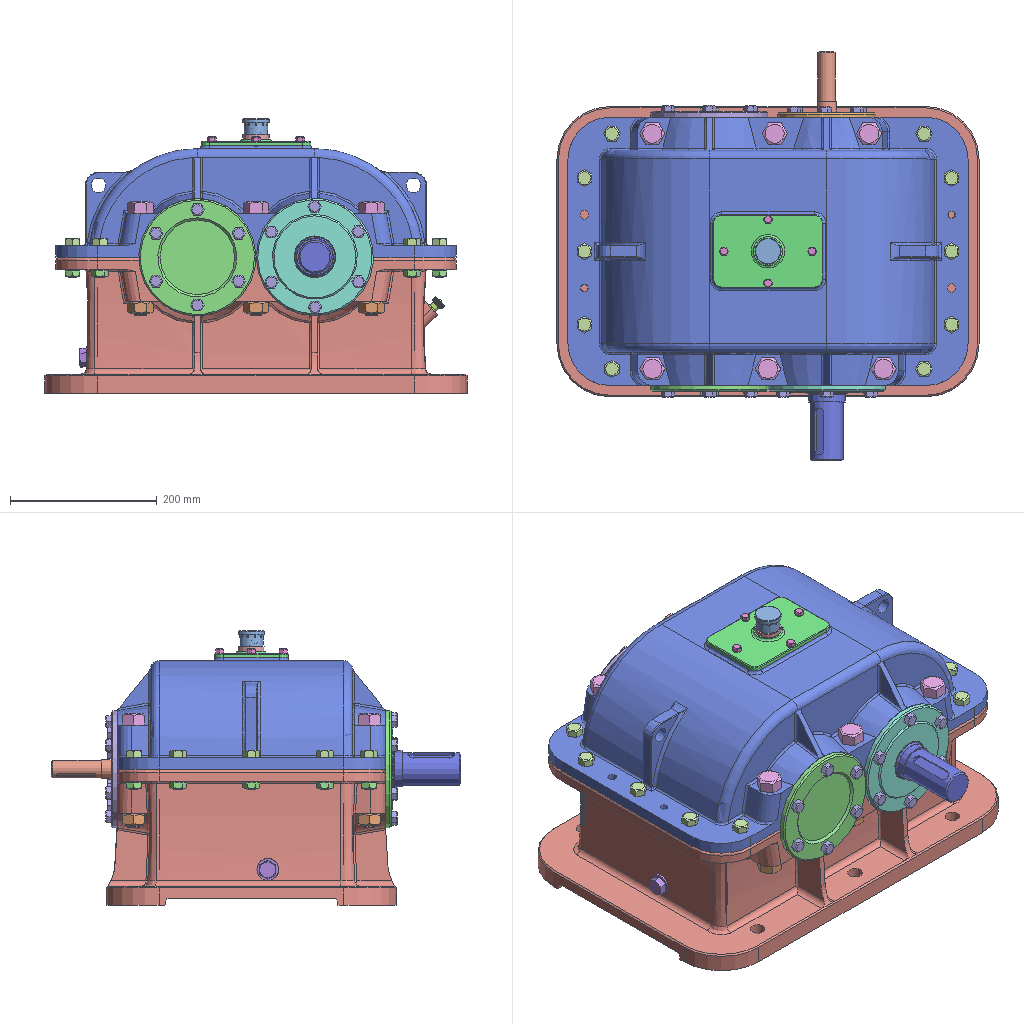Assembly | NX | 39 different items | 103 placed | box 576 x 558 x 375 mm
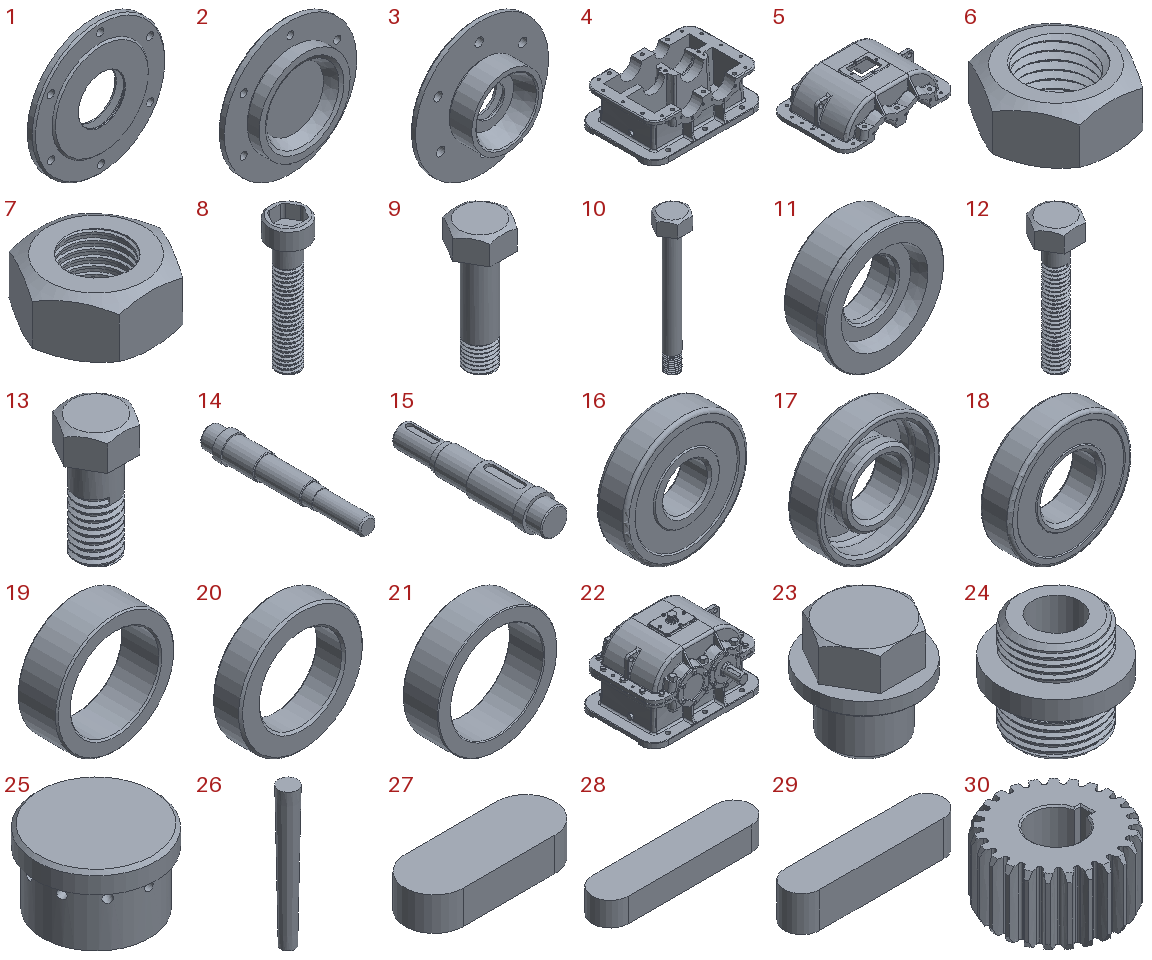Parts list (item | quantity | parent item | size | volume | features):
1 | x1 | in 22 | 160 x 18 x 160 mm | 177921 mm3 | features BREP 1, DATUM_CSYS 1
2 | x1 | in 22 | 160 x 25 x 160 mm | 214879 mm3 | features BREP 1, DATUM_CSYS 1
3 | x1 | in 22 | 135 x 31.5 x 135 mm | 118525 mm3 | features BREP 1, DATUM_CSYS 1
4 | x1 | in 22 | 576 x 396 x 186 mm | 12365991 mm3 | features DATUM_CSYS 8, SKETCH 7, EXTRUDE 6, BLEND 2, DATUM_PLANE 2, THREADS 2, BREP 1
5 | x1 | in 22 | - | - | features BLEND 4, DATUM_CSYS 3, EXTRUDE 3, SKETCH 2, BREP 1, CPROJ 1, DATUM_PLANE 1
6 | x10 | in 22 | 23.094 x 20 x 10 mm | 1985 mm3 | features DATUM_CSYS 3, SKETCH 2, EXTRUDE 1, SWP104 1, THREADS 1
7 | x6 | in 22 | 34.641 x 30 x 16 mm | 8595 mm3 | features DATUM_CSYS 3, SKETCH 2, EXTRUDE 1, SWP104 1, THREADS 1
8 | x2 | in 22 | 20 x 20 x 70 mm | 7911 mm3 | features DATUM_CSYS 3, EXTRUDE 2, SKETCH 2, BLEND 1, CHAMFER 1, CYLINDER 1, THREADS 1
9 | x10 | in 22 | - | - | features DATUM_CSYS 3, SKETCH 2, CYLINDER 1, EXTRUDE 1, SWP104 1, THREADS 1
10 | x6 | in 22 | 34.641 x 30 x 156 mm | 39944 mm3 | features DATUM_CSYS 3, SKETCH 2, CYLINDER 1, EXTRUDE 1, SWP104 1, THREADS 1
11 | x1 | in 22 | 130 x 50.5 x 130 mm | 363881 mm3 | features BREP 1, DATUM_CSYS 1
12 | x24 | in 22 | 18.475 x 16 x 56 mm | 4007 mm3 | features DATUM_CSYS 3, SKETCH 2, CYLINDER 1, EXTRUDE 1, SWP104 1, THREADS 1
13 | x4 | in 22 | - | - | features DATUM_CSYS 3, SKETCH 2, CYLINDER 1, EXTRUDE 1, SWP104 1, THREADS 1
14 | x1 | in 22 | 38 x 227.5 x 38 mm | 152701 mm3 | features DATUM_CSYS 4, SKETCH 3, CHAMFER 2, DATUM_PLANE 2, EXTRUDE 2, CPROJ 1, SWP104 1
15 | x1 | in 22 | 68 x 312 x 68 mm | 761578 mm3 | features DATUM_CSYS 4, CHAMFER 3, SKETCH 3, DATUM_PLANE 2, EXTRUDE 2, SWP104 1
16 | x2 | in 22 | 110 x 27 x 110 mm | 123017 mm3 | features BREP 1, DATUM_CSYS 1
17 | x2 | in 22 | 72 x 19 x 72 mm | 32783 mm3 | features BREP 1, DATUM_CSYS 1
18 | x2 | in 22 | 120 x 29 x 120 mm | 129024 mm3 | features BREP 1, DATUM_CSYS 1
19 | x1 | - | 40 x 13.5 x 40 mm | 7367 mm3 | features BREP 1, DATUM_CSYS 1
20 | x1 | - | 60 x 14 x 60 mm | 21677 mm3 | features BREP 1, DATUM_CSYS 1
21 | x1 | - | 71 x 21 x 71 mm | 33152 mm3 | features BREP 1, DATUM_CSYS 1
22 | x1 | - | - | 23332165 mm3 | features BREP 221, META 208, DATUM_CSYS 102, SWP104 95, EXTRACT_STRING 92, Instance Feature 88, SKETCH 68, EXTRUDE 61, CHAMFER 19, BLEND 12, CYLINDER 10, DATUM_PLANE 10, THREADS 9, CPROJ 7, BOSS 4, FSET 4, Pattern Feature 3, Mirror Feature 1, WRAP 1
23 | x1 | in 22 | 30 x 30 x 29 mm | 11364 mm3 | features DATUM_CSYS 4, SKETCH 3, CHAMFER 2, SWP104 2, DATUM_PLANE 1, EXTRUDE 1
24 | x1 | in 22 | 36 x 36 x 32 mm | 13512 mm3 | features BREP 1, DATUM_CSYS 1
25 | x1 | in 22 | 36 x 36 x 22 mm | 11377 mm3 | features EXTRUDE 12, EXTRACT_STRING 10, Instance Feature 9, DATUM_CSYS 4, SKETCH 3, BOSS 1, CHAMFER 1, CYLINDER 1, Pattern Feature 1
26 | x2 | in 22 | 8.095 x 8.095 x 60 mm | 2358 mm3 | features DATUM_CSYS 2, EXTRUDE 1, SKETCH 1
27 | x1 | in 22 | 36 x 14 x 8 mm | 3696 mm3 | features DATUM_CSYS 2, EXTRUDE 1, SKETCH 1
28 | x1 | in 22 | 80 x 18 x 12 mm | 16446 mm3 | features DATUM_CSYS 2, EXTRUDE 1, SKETCH 1
29 | x1 | in 22 | 36 x 8 x 8 mm | 2194 mm3 | features DATUM_CSYS 2, EXTRUDE 1, SKETCH 1
30 | x1 | in 22 | 83.645 x 83.495 x 45 mm | 166384 mm3 | features BREP 25, META 25, DATUM_CSYS 4, SKETCH 3, EXTRUDE 2, CHAMFER 1, CPROJ 1, CYLINDER 1, FSET 1, SWP104 1
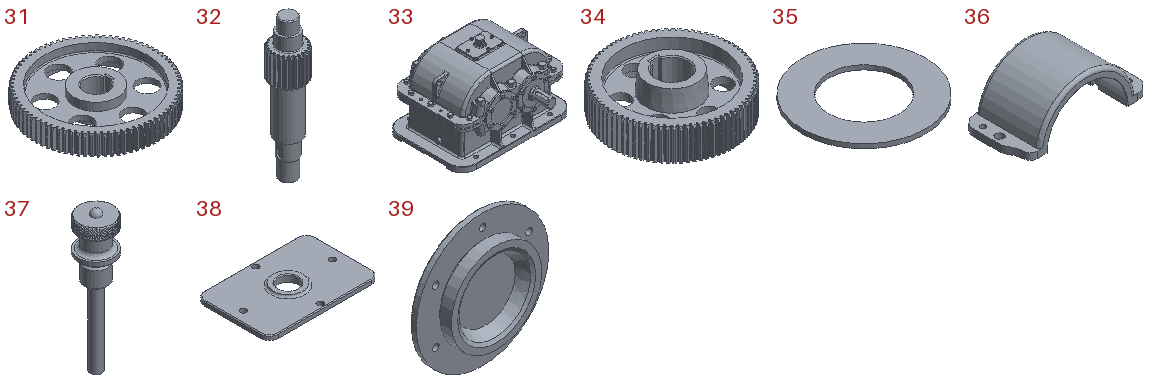31 | x1 | in 22 | 247.038 x 246.995 x 40 mm | 857249 mm3 | features BREP 79, META 79, DATUM_CSYS 7, SKETCH 6, EXTRUDE 5, CPROJ 2, BLEND 1, CHAMFER 1, CYLINDER 1, FSET 1, SWP104 1
32 | x1 | in 22 | 82.296 x 82.148 x 342.25 mm | 879629 mm3 | features BREP 25, META 25, DATUM_CSYS 5, SKETCH 4, BOSS 3, EXTRUDE 3, CHAMFER 2, BLEND 1, CYLINDER 1, FSET 1, SWP104 1
33 | x1 | - | - | 23332165 mm3 | features BREP 221, META 208, DATUM_CSYS 102, SWP104 95, EXTRACT_STRING 92, Instance Feature 88, SKETCH 68, EXTRUDE 61, CHAMFER 19, BLEND 12, CYLINDER 10, DATUM_PLANE 10, THREADS 9, CPROJ 7, BOSS 4, FSET 4, Pattern Feature 3, Mirror Feature 1, WRAP 1
34 | x1 | in 22 | 247.038 x 246.995 x 94 mm | 1592670 mm3 | features BREP 79, META 79, DATUM_CSYS 10, SKETCH 9, EXTRUDE 8, BLEND 1, CHAMFER 1, CPROJ 1, CYLINDER 1, FSET 1, SWP104 1
35 | x6 | in 22 | 28 x 28 x 1 mm | 414.69 mm3 | features DATUM_CSYS 2, EXTRUDE 1, SKETCH 1
36 | x1 | in 22 | 190 x 95 x 73.244 mm | 279574 mm3 | features BREP 1, CHAMFER 1, DATUM_CSYS 1, DATUM_PLANE 1
37 | x1 | in 22 | 18 x 18 x 72.5 mm | 5643 mm3 | features EXTRACT_STRING 82, SWP104 81, Instance Feature 79, DATUM_CSYS 4, CHAMFER 3, SKETCH 3, Pattern Feature 2, BLEND 1, DATUM_PLANE 1, Mirror Feature 1, WRAP 1
38 | x1 | in 22 | 150 x 100 x 10 mm | 75362 mm3 | features DATUM_CSYS 2, BLEND 1, BREP 1, CHAMFER 1, CPROJ 1, EXTRUDE 1, SKETCH 1
39 | x1 | in 22 | 160 x 25 x 160 mm | 214093 mm3 | features DATUM_CSYS 3, EXTRUDE 3, SKETCH 2, BREP 1
Mates (type | each side: item.copy, entity, surface, feature):
Fix | 4.1 component
Concentric | 4.1 edge | 5.1 edge
Parallel | 5.1 face plane Body(1) | 4.1 face plane Body(1)
Concentric | 3.1 edge | 5.1 edge | 2 times
Concentric | 5.1 edge | 1.1 edge | 2 times
Concentric | 5.1 edge | 39.1 edge
Distance | 39.1 face cylinder Extrude(6) | 5.1 face cylinder Body(1)
Concentric | 5.1 edge | 2.1 edge
Distance | 2.1 face cylinder Body(1) | 5.1 face cylinder Body(1)
Concentric | 11.1 edge | 4.1 edge
Concentric | 2.1 edge | 16.1 edge
Concentric | 16.1 edge | 39.1 edge
Concentric | 17.1 edge | 3.1 edge
Concentric | 1.1 edge | 18.1 edge
Concentric | 18.1 edge | 11.1 edge
Concentric | 4.1 edge | 36.1 edge
Parallel | 36.1 face plane Body(1) | 11.1 face plane Body(1)
Concentric | 17.1 edge | 11.1 edge
Touch | 14.1 face cylinder Revolve(2) | 3.1 face cylinder Body(1)
Distance | 14.1 face plane Revolve(2) | 3.1 face plane Body(1)
Touch | 15.1 face cylinder Revolve(2) | 18.1 face cone Body(1)
Distance | 15.1 face plane Revolve(2) | 1.1 face plane Body(1)
Parallel | 30.1 face plane Extrude(56) | 14.1 face plane Extrude(7)
Touch | 30.1 face cylinder Extrude(54) | 14.1 face cylinder Revolve(2)
Center22 | 30.1 face plane Cylinder(1) | 30.1 face plane Cylinder(1) | 4.1 face plane Body(1) | 11.1 face plane Body(1)
Touch | 31.1 face cylinder Extrude(166) | 16.1 face cylinder Body(1)
Center22 | 31.1 face plane Cylinder(1) | 31.1 face plane Cylinder(1) | 30.1 face plane Cylinder(1) | 30.1 face plane Cylinder(1)
Parallel | 32.1 face plane Extrude(64) | 31.1 face plane Extrude(164)
Parallel | 34.1 face plane Extrude(174) | 15.1 face plane Extrude(7)
Touch | 34.1 face cylinder Extrude(162) | 15.1 face cylinder Revolve(2)
Center22 | 34.1 face plane Cylinder(1) | 34.1 face plane Cylinder(1) | 32.1 face plane Cylinder(1) | 32.1 face plane Cylinder(1)
Concentric | 23.1 edge | 4.1 edge
Distance | 4.1 face plane Body(1) | 32.1 face plane Cylinder(1)
Distance | 32.1 face cylinder Extrude(58) | 4.1 face plane Body(1) | 2 times
Concentric | 5.1 edge | 38.1 edge
Parallel | 38.1 face plane Body(1) | 5.1 face plane Body(1)
Concentric | 24.1 edge | 38.1 edge
Concentric | 25.1 edge | 24.1 edge
Concentric | 37.1 edge | 4.1 edge
Concentric | 5.1 edge | 10.1 edge | 5 times
Parallel | 10.1 face plane Extrude(4) | 3.1 face plane Body(1) | 2 times
Parallel | 10.1 face plane Extrude(4) | 39.1 face plane Body(1)
Parallel | 10.1 face plane Extrude(4) | 1.1 face plane Body(1)
Parallel | 10.1 face plane Extrude(4) | 5.1 face plane Body(1)
Concentric | 5.1 edge | 10.1
Parallel | 10.1 | 2.1 face plane Body(1)
Concentric | 35.1 | 4.1 edge | 4 times
Concentric | 35.1 edge | 4.1 edge | 2 times
Concentric | 7.1 arc | 35.1 | 4 times
Parallel | 7.1 face plane Extrude(2) | 3.1 face plane Body(1)
Concentric | 7.1 arc | 35.1 edge | 2 times
Parallel | 7.1 face plane Extrude(2) | 4.1 face plane Body(1)
Parallel | 7.1 face plane Extrude(2) | 39.1 face plane Body(1)
Parallel | 7.1 face plane Extrude(2) | 1.1 face plane Body(1)
Parallel | 7.1 | 2.1 face plane Body(1) | 2 times
Concentric | 2.1 edge | 12.1
Parallel | 12.1 | 5.1 face plane Body(1)
Fix | 22.1 component | 4 times
Bond | 12.1 component | 22.1 component | 24 times
CircularPattern | 22.2 axis | 22.2 csys | 22.2 csys | 22.2 csys | 22.2 csys | 22.2 csys | 22.2 csys | 4 times
Concentric | 1.1 edge | 12.1 edge
Parallel | 12.1 face plane Extrude(3) | 5.1 face plane Body(1) | 3 times
Concentric | 39.1 edge | 12.1 edge
Concentric | 3.1 edge | 12.1 edge
Concentric | 5.1 edge | 9.1 edge | 4 times
Parallel | 9.1 face plane Extrude(3) | 5.1 face plane Body(1) | 4 times
Concentric | 5.1 edge | 9.1 | 6 times
Parallel | 9.1 | 5.1 face plane Body(1) | 5 times
Concentric | 6.1 arc | 4.1 edge | 4 times
Parallel | 6.1 | 4.1 face plane Body(1) | 8 times
Concentric | 6.1 | 4.1 edge | 4 times
Parallel | 6.1 face plane Extrude(2) | 4.1 face plane Body(1) | 2 times
Parallel | 9.1 | 4.1 edge
Concentric | 4.1 edge | 6.1
Concentric | 38.1 edge | 13.1 | 3 times
Parallel | 13.1 | 38.1 face plane Body(1) | 3 times
Concentric | 38.1 edge | 13.1 edge
Parallel | 13.1 face plane Extrude(3) | 38.1 face plane Body(1)
Concentric | 6.1 edge | 4.1 edge
Concentric | 36.1 edge | 8.1 arc
Concentric | 8.1 arc | 36.1 edge
Concentric | 26.1 arc | 4.1 edge | 2 times
Concentric | 29.1 arc | 14.1 edge
Parallel | 29.1 face plane Extrude(2) | 14.1 face plane Extrude(7)
Concentric | 27.1 arc | 32.1 edge
Parallel | 27.1 | 32.1 face plane Extrude(64)
Concentric | 15.1 edge | 28.1 arc
Parallel | 28.1 | 15.1 face plane Extrude(7)